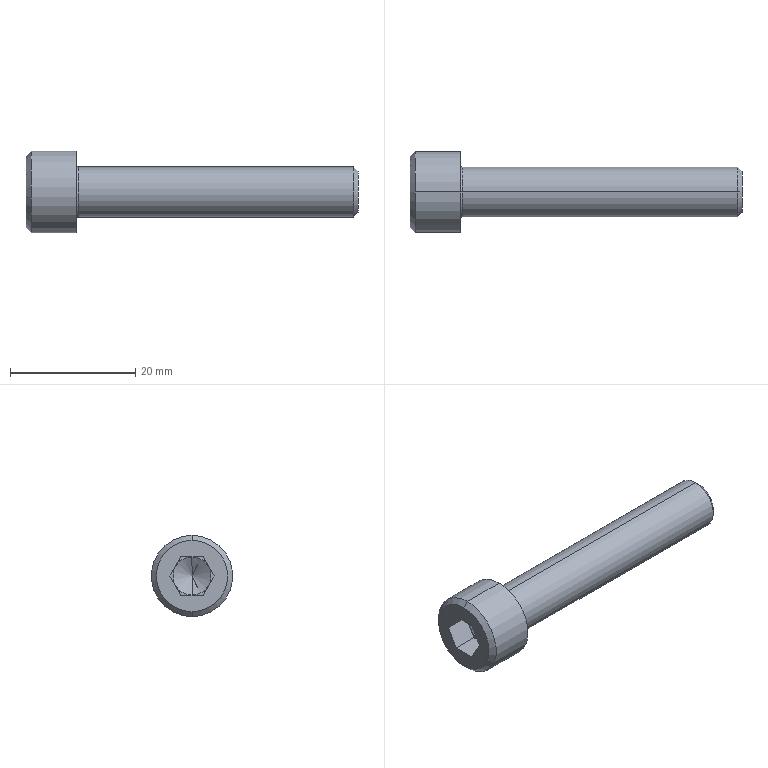Part | SolidWorks | features CirPattern 3, Cut 3, RevCut 2, Fillet 1, LPattern 1, Revolution 1 | 1 solid | 27 faces | box 53 x 13 x 13 mm | volume 3161 mm3 | plane 15 | cone 6 | cylinder 4 | torus 2 | commonest cylinder face diameters 8 x2 13 x2
STEP:
#1=CARTESIAN_POINT('',(5.759,0.,0.));
#2=VERTEX_POINT('',#1);
#3=CARTESIAN_POINT('',(4.,0.,3.047));
#4=VERTEX_POINT('',#3);
#5=CARTESIAN_POINT('',(4.,0.,3.048));
#6=DIRECTION('',(-0.5,0.,0.866));
#7=VECTOR('',#6,1000.);
#8=LINE('',#5,#7);
#9=EDGE_CURVE('',#2,#4,#8,.T.);
#10=ORIENTED_EDGE('',*,*,#9,.F.);
#11=CARTESIAN_POINT('',(4.,0.,-3.047));
#12=VERTEX_POINT('',#11);
#13=CARTESIAN_POINT('',(4.,0.,-3.048));
#14=DIRECTION('',(-0.5,0.,-0.866));
#15=VECTOR('',#14,1000.);
#16=LINE('',#13,#15);
#17=EDGE_CURVE('',#2,#12,#16,.T.);
#18=ORIENTED_EDGE('',*,*,#17,.T.);
#19=CARTESIAN_POINT('',(4.,-2.639,-1.524));
#20=VERTEX_POINT('',#19);
#21=CARTESIAN_POINT('',(4.,0.,0.));
#22=DIRECTION('',(-1.,0.,0.));
#23=DIRECTION('',(0.,0.,1.));
#24=AXIS2_PLACEMENT_3D('',#21,#22,#23);
#25=CIRCLE('',#24,3.048);
#26=EDGE_CURVE('',#12,#20,#25,.T.);
#27=ORIENTED_EDGE('',*,*,#26,.T.);
#28=CARTESIAN_POINT('',(4.,-2.639,1.524));
#29=VERTEX_POINT('',#28);
#30=CARTESIAN_POINT('',(4.,0.,0.));
#31=DIRECTION('',(-1.,0.,0.));
#32=DIRECTION('',(0.,0.,1.));
#33=AXIS2_PLACEMENT_3D('',#30,#31,#32);
#34=CIRCLE('',#33,3.048);
#35=EDGE_CURVE('',#20,#29,#34,.T.);
#36=ORIENTED_EDGE('',*,*,#35,.T.);
#37=CARTESIAN_POINT('',(4.,0.,0.));
#38=DIRECTION('',(-1.,0.,0.));
#39=DIRECTION('',(0.,0.,1.));
#40=AXIS2_PLACEMENT_3D('',#37,#38,#39);
#41=CIRCLE('',#40,3.048);
#42=EDGE_CURVE('',#29,#4,#41,.T.);
#43=ORIENTED_EDGE('',*,*,#42,.T.);
#44=EDGE_LOOP('',(#10,#18,#27,#36,#43));
#45=FACE_OUTER_BOUND('',#44,.T.);
#46=CARTESIAN_POINT('',(4.,0.,0.));
#47=DIRECTION('',(-1.,0.,0.));
#48=DIRECTION('',(0.,0.,1.));
#49=AXIS2_PLACEMENT_3D('',#46,#47,#48);
#50=CONICAL_SURFACE('',#49,3.048,1.047);
#51=ADVANCED_FACE('',(#45),#50,.F.);
#52=CARTESIAN_POINT('',(8.4,0.,4.));
#53=VERTEX_POINT('',#52);
#54=CARTESIAN_POINT('',(8.4,0.,-4.));
#55=VERTEX_POINT('',#54);
#56=CARTESIAN_POINT('',(8.4,0.,0.));
#57=DIRECTION('',(1.,0.,0.));
#58=DIRECTION('',(0.,0.,-1.));
#59=AXIS2_PLACEMENT_3D('',#56,#57,#58);
#60=CIRCLE('',#59,4.);
#61=EDGE_CURVE('',#53,#55,#60,.T.);
#62=ORIENTED_EDGE('',*,*,#61,.F.);
#63=CARTESIAN_POINT('',(8.,0.,4.4));
#64=VERTEX_POINT('',#63);
#65=CARTESIAN_POINT('',(8.4,0.,4.4));
#66=DIRECTION('',(0.,1.,0.));
#67=DIRECTION('',(0.,0.,1.));
#68=AXIS2_PLACEMENT_3D('',#65,#66,#67);
#69=CIRCLE('',#68,0.4);
#70=EDGE_CURVE('',#53,#64,#69,.T.);
#71=ORIENTED_EDGE('',*,*,#70,.T.);
#72=CARTESIAN_POINT('',(8.,0.,-4.4));
#73=VERTEX_POINT('',#72);
#74=CARTESIAN_POINT('',(8.,0.,0.));
#75=DIRECTION('',(-1.,0.,0.));
#76=DIRECTION('',(0.,0.,-1.));
#77=AXIS2_PLACEMENT_3D('',#74,#75,#76);
#78=CIRCLE('',#77,4.4);
#79=EDGE_CURVE('',#73,#64,#78,.T.);
#80=ORIENTED_EDGE('',*,*,#79,.F.);
#81=CARTESIAN_POINT('',(8.4,0.,-4.4));
#82=DIRECTION('',(0.,-1.,0.));
#83=DIRECTION('',(0.,0.,-1.));
#84=AXIS2_PLACEMENT_3D('',#81,#82,#83);
#85=CIRCLE('',#84,0.4);
#86=EDGE_CURVE('',#55,#73,#85,.T.);
#87=ORIENTED_EDGE('',*,*,#86,.F.);
#88=EDGE_LOOP('',(#62,#71,#80,#87));
#89=FACE_OUTER_BOUND('',#88,.T.);
#90=CARTESIAN_POINT('',(8.4,0.,0.));
#91=DIRECTION('',(1.,0.,0.));
#92=DIRECTION('',(0.,0.,-1.));
#93=AXIS2_PLACEMENT_3D('',#90,#91,#92);
#94=TOROIDAL_SURFACE('',#93,4.4,0.4);
#95=ADVANCED_FACE('',(#89),#94,.F.);
#96=CARTESIAN_POINT('',(0.,0.,5.7));
#97=VERTEX_POINT('',#96);
#98=CARTESIAN_POINT('',(0.,0.,-5.7));
#99=VERTEX_POINT('',#98);
#100=CARTESIAN_POINT('',(0.,0.,0.));
#101=DIRECTION('',(-1.,0.,0.));
#102=DIRECTION('',(0.,0.,1.));
#103=AXIS2_PLACEMENT_3D('',#100,#101,#102);
#104=CIRCLE('',#103,5.7);
#105=EDGE_CURVE('',#97,#99,#104,.T.);
#106=ORIENTED_EDGE('',*,*,#105,.F.);
#107=CARTESIAN_POINT('',(0.8,0.,6.5));
#108=VERTEX_POINT('',#107);
#109=CARTESIAN_POINT('',(0.,0.,5.7));
#110=DIRECTION('',(0.7071,0.,0.7071));
#111=VECTOR('',#110,1000.);
#112=LINE('',#109,#111);
#113=EDGE_CURVE('',#97,#108,#112,.T.);
#114=ORIENTED_EDGE('',*,*,#113,.T.);
#115=CARTESIAN_POINT('',(0.8,0.,-6.5));
#116=VERTEX_POINT('',#115);
#117=CARTESIAN_POINT('',(0.8,0.,0.));
#118=DIRECTION('',(-1.,0.,0.));
#119=DIRECTION('',(0.,0.,1.));
#120=AXIS2_PLACEMENT_3D('',#117,#118,#119);
#121=CIRCLE('',#120,6.5);
#122=EDGE_CURVE('',#108,#116,#121,.T.);
#123=ORIENTED_EDGE('',*,*,#122,.T.);
#124=CARTESIAN_POINT('',(0.,0.,-5.7));
#125=DIRECTION('',(0.7071,0.,-0.7071));
#126=VECTOR('',#125,1000.);
#127=LINE('',#124,#126);
#128=EDGE_CURVE('',#99,#116,#127,.T.);
#129=ORIENTED_EDGE('',*,*,#128,.F.);
#130=EDGE_LOOP('',(#106,#114,#123,#129));
#131=FACE_OUTER_BOUND('',#130,.T.);
#132=CARTESIAN_POINT('',(0.,0.,0.));
#133=DIRECTION('',(1.,0.,0.));
#134=DIRECTION('',(0.,0.,-1.));
#135=AXIS2_PLACEMENT_3D('',#132,#133,#134);
#136=CONICAL_SURFACE('',#135,5.7,0.7854);
#137=ADVANCED_FACE('',(#131),#136,.T.);
#138=CARTESIAN_POINT('',(8.,0.,6.5));
#139=VERTEX_POINT('',#138);
#140=CARTESIAN_POINT('',(8.,0.,-6.5));
#141=VERTEX_POINT('',#140);
#142=CARTESIAN_POINT('',(8.,0.,0.));
#143=DIRECTION('',(-1.,0.,0.));
#144=DIRECTION('',(0.,0.,1.));
#145=AXIS2_PLACEMENT_3D('',#142,#143,#144);
#146=CIRCLE('',#145,6.5);
#147=EDGE_CURVE('',#139,#141,#146,.T.);
#148=ORIENTED_EDGE('',*,*,#147,.T.);
#149=CARTESIAN_POINT('',(-31.75,0.,-6.5));
#150=DIRECTION('',(-1.,0.,0.));
#151=VECTOR('',#150,1000.);
#152=LINE('',#149,#151);
#153=EDGE_CURVE('',#141,#116,#152,.T.);
#154=ORIENTED_EDGE('',*,*,#153,.T.);
#155=ORIENTED_EDGE('',*,*,#122,.F.);
#156=CARTESIAN_POINT('',(-31.75,0.,6.5));
#157=DIRECTION('',(-1.,0.,0.));
#158=VECTOR('',#157,1000.);
#159=LINE('',#156,#158);
#160=EDGE_CURVE('',#139,#108,#159,.T.);
#161=ORIENTED_EDGE('',*,*,#160,.F.);
#162=EDGE_LOOP('',(#148,#154,#155,#161));
#163=FACE_OUTER_BOUND('',#162,.T.);
#164=CARTESIAN_POINT('',(-31.75,0.,0.));
#165=DIRECTION('',(-1.,0.,0.));
#166=DIRECTION('',(0.,0.,1.));
#167=AXIS2_PLACEMENT_3D('',#164,#165,#166);
#168=CYLINDRICAL_SURFACE('',#167,6.5);
#169=ADVANCED_FACE('',(#163),#168,.T.);
#170=CARTESIAN_POINT('',(52.31,0.,4.));
#171=VERTEX_POINT('',#170);
#172=CARTESIAN_POINT('',(52.31,0.,-4.));
#173=VERTEX_POINT('',#172);
#174=CARTESIAN_POINT('',(52.31,0.,0.));
#175=DIRECTION('',(-1.,0.,0.));
#176=DIRECTION('',(0.,0.,1.));
#177=AXIS2_PLACEMENT_3D('',#174,#175,#176);
#178=CIRCLE('',#177,4.);
#179=EDGE_CURVE('',#171,#173,#178,.T.);
#180=ORIENTED_EDGE('',*,*,#179,.T.);
#181=CARTESIAN_POINT('',(-31.75,0.,-4.));
#182=DIRECTION('',(-1.,0.,0.));
#183=VECTOR('',#182,1000.);
#184=LINE('',#181,#183);
#185=EDGE_CURVE('',#173,#55,#184,.T.);
#186=ORIENTED_EDGE('',*,*,#185,.T.);
#187=CARTESIAN_POINT('',(8.4,0.,0.));
#188=DIRECTION('',(1.,0.,0.));
#189=DIRECTION('',(0.,0.,-1.));
#190=AXIS2_PLACEMENT_3D('',#187,#188,#189);
#191=CIRCLE('',#190,4.);
#192=EDGE_CURVE('',#55,#53,#191,.T.);
#193=ORIENTED_EDGE('',*,*,#192,.T.);
#194=CARTESIAN_POINT('',(-31.75,0.,4.));
#195=DIRECTION('',(-1.,0.,0.));
#196=VECTOR('',#195,1000.);
#197=LINE('',#194,#196);
#198=EDGE_CURVE('',#171,#53,#197,.T.);
#199=ORIENTED_EDGE('',*,*,#198,.F.);
#200=EDGE_LOOP('',(#180,#186,#193,#199));
#201=FACE_OUTER_BOUND('',#200,.T.);
#202=CARTESIAN_POINT('',(-31.75,0.,0.));
#203=DIRECTION('',(-1.,0.,0.));
#204=DIRECTION('',(0.,0.,1.));
#205=AXIS2_PLACEMENT_3D('',#202,#203,#204);
#206=CYLINDRICAL_SURFACE('',#205,4.);
#207=ADVANCED_FACE('',(#201),#206,.T.);
#208=CARTESIAN_POINT('',(53.,0.,3.309));
#209=VERTEX_POINT('',#208);
#210=CARTESIAN_POINT('',(53.,0.,-3.309));
#211=VERTEX_POINT('',#210);
#212=CARTESIAN_POINT('',(53.,0.,0.));
#213=DIRECTION('',(-1.,0.,0.));
#214=DIRECTION('',(0.,0.,1.));
#215=AXIS2_PLACEMENT_3D('',#212,#213,#214);
#216=CIRCLE('',#215,3.309);
#217=EDGE_CURVE('',#209,#211,#216,.T.);
#218=ORIENTED_EDGE('',*,*,#217,.T.);
#219=CARTESIAN_POINT('',(53.,0.,-3.309));
#220=DIRECTION('',(-0.7071,0.,-0.7071));
#221=VECTOR('',#220,1000.);
#222=LINE('',#219,#221);
#223=EDGE_CURVE('',#211,#173,#222,.T.);
#224=ORIENTED_EDGE('',*,*,#223,.T.);
#225=ORIENTED_EDGE('',*,*,#179,.F.);
#226=CARTESIAN_POINT('',(53.,0.,3.309));
#227=DIRECTION('',(-0.7071,0.,0.7071));
#228=VECTOR('',#227,1000.);
#229=LINE('',#226,#228);
#230=EDGE_CURVE('',#209,#171,#229,.T.);
#231=ORIENTED_EDGE('',*,*,#230,.F.);
#232=EDGE_LOOP('',(#218,#224,#225,#231));
#233=FACE_OUTER_BOUND('',#232,.T.);
#234=CARTESIAN_POINT('',(53.,0.,0.));
#235=DIRECTION('',(-1.,0.,0.));
#236=DIRECTION('',(0.,0.,1.));
#237=AXIS2_PLACEMENT_3D('',#234,#235,#236);
#238=CONICAL_SURFACE('',#237,3.309,0.7854);
#239=ADVANCED_FACE('',(#233),#238,.T.);
#240=CARTESIAN_POINT('',(0.,3.519,0.));
#241=VERTEX_POINT('',#240);
#242=CARTESIAN_POINT('',(0.,1.759,3.047));
#243=VERTEX_POINT('',#242);
#244=CARTESIAN_POINT('',(0.,3.519,0.));
#245=DIRECTION('',(0.,-0.5,0.866));
#246=VECTOR('',#245,1000.);
#247=LINE('',#244,#246);
#248=EDGE_CURVE('',#241,#243,#247,.T.);
#249=ORIENTED_EDGE('',*,*,#248,.T.);
#250=CARTESIAN_POINT('',(0.,-1.759,3.048));
#251=VERTEX_POINT('',#250);
#252=CARTESIAN_POINT('',(0.,-1.759,3.048));
#253=DIRECTION('',(0.,1.,0.));
#254=VECTOR('',#253,1000.);
#255=LINE('',#252,#254);
#256=EDGE_CURVE('',#251,#243,#255,.T.);
#257=ORIENTED_EDGE('',*,*,#256,.F.);
#258=CARTESIAN_POINT('',(0.,-3.519,0.));
#259=VERTEX_POINT('',#258);
#260=CARTESIAN_POINT('',(0.,-1.759,3.048));
#261=DIRECTION('',(0.,-0.5,-0.866));
#262=VECTOR('',#261,1000.);
#263=LINE('',#260,#262);
#264=EDGE_CURVE('',#251,#259,#263,.T.);
#265=ORIENTED_EDGE('',*,*,#264,.T.);
#266=CARTESIAN_POINT('',(0.,-1.759,-3.047));
#267=VERTEX_POINT('',#266);
#268=CARTESIAN_POINT('',(0.,-3.519,0.));
#269=DIRECTION('',(0.,0.5,-0.866));
#270=VECTOR('',#269,1000.);
#271=LINE('',#268,#270);
#272=EDGE_CURVE('',#259,#267,#271,.T.);
#273=ORIENTED_EDGE('',*,*,#272,.T.);
#274=CARTESIAN_POINT('',(0.,1.759,-3.048));
#275=VERTEX_POINT('',#274);
#276=CARTESIAN_POINT('',(0.,1.759,-3.048));
#277=DIRECTION('',(0.,-1.,0.));
#278=VECTOR('',#277,1000.);
#279=LINE('',#276,#278);
#280=EDGE_CURVE('',#275,#267,#279,.T.);
#281=ORIENTED_EDGE('',*,*,#280,.F.);
#282=CARTESIAN_POINT('',(0.,3.519,0.));
#283=DIRECTION('',(0.,-0.5,-0.866));
#284=VECTOR('',#283,1000.);
#285=LINE('',#282,#284);
#286=EDGE_CURVE('',#241,#275,#285,.T.);
#287=ORIENTED_EDGE('',*,*,#286,.F.);
#288=EDGE_LOOP('',(#249,#257,#265,#273,#281,#287));
#289=FACE_BOUND('',#288,.T.);
#290=CARTESIAN_POINT('',(0.,0.,0.));
#291=DIRECTION('',(-1.,0.,0.));
#292=DIRECTION('',(0.,0.,1.));
#293=AXIS2_PLACEMENT_3D('',#290,#291,#292);
#294=CIRCLE('',#293,5.7);
#295=EDGE_CURVE('',#99,#97,#294,.T.);
#296=ORIENTED_EDGE('',*,*,#295,.T.);
#297=ORIENTED_EDGE('',*,*,#105,.T.);
#298=EDGE_LOOP('',(#296,#297));
#299=FACE_OUTER_BOUND('',#298,.T.);
#300=CARTESIAN_POINT('',(0.,0.,0.));
#301=DIRECTION('',(-1.,0.,0.));
#302=DIRECTION('',(0.,0.,1.));
#303=AXIS2_PLACEMENT_3D('',#300,#301,#302);
#304=PLANE('',#303);
#305=ADVANCED_FACE('',(#289,#299),#304,.T.);
#306=ORIENTED_EDGE('',*,*,#217,.F.);
#307=CARTESIAN_POINT('',(53.,0.,0.));
#308=DIRECTION('',(-1.,0.,0.));
#309=DIRECTION('',(0.,0.,1.));
#310=AXIS2_PLACEMENT_3D('',#307,#308,#309);
#311=CIRCLE('',#310,3.309);
#312=EDGE_CURVE('',#211,#209,#311,.T.);
#313=ORIENTED_EDGE('',*,*,#312,.F.);
#314=EDGE_LOOP('',(#306,#313));
#315=FACE_OUTER_BOUND('',#314,.T.);
#316=CARTESIAN_POINT('',(53.,3.309,0.));
#317=DIRECTION('',(1.,0.,0.));
#318=DIRECTION('',(0.,0.,-1.));
#319=AXIS2_PLACEMENT_3D('',#316,#317,#318);
#320=PLANE('',#319);
#321=ADVANCED_FACE('',(#315),#320,.T.);
#322=ORIENTED_EDGE('',*,*,#223,.F.);
#323=ORIENTED_EDGE('',*,*,#312,.T.);
#324=ORIENTED_EDGE('',*,*,#230,.T.);
#325=CARTESIAN_POINT('',(52.31,0.,0.));
#326=DIRECTION('',(-1.,0.,0.));
#327=DIRECTION('',(0.,0.,1.));
#328=AXIS2_PLACEMENT_3D('',#325,#326,#327);
#329=CIRCLE('',#328,4.);
#330=EDGE_CURVE('',#173,#171,#329,.T.);
#331=ORIENTED_EDGE('',*,*,#330,.F.);
#332=EDGE_LOOP('',(#322,#323,#324,#331));
#333=FACE_OUTER_BOUND('',#332,.T.);
#334=CARTESIAN_POINT('',(53.,0.,0.));
#335=DIRECTION('',(-1.,0.,0.));
#336=DIRECTION('',(0.,0.,1.));
#337=AXIS2_PLACEMENT_3D('',#334,#335,#336);
#338=CONICAL_SURFACE('',#337,3.309,0.7854);
#339=ADVANCED_FACE('',(#333),#338,.T.);
#340=ORIENTED_EDGE('',*,*,#185,.F.);
#341=ORIENTED_EDGE('',*,*,#330,.T.);
#342=ORIENTED_EDGE('',*,*,#198,.T.);
#343=ORIENTED_EDGE('',*,*,#61,.T.);
#344=EDGE_LOOP('',(#340,#341,#342,#343));
#345=FACE_OUTER_BOUND('',#344,.T.);
#346=CARTESIAN_POINT('',(-31.75,0.,0.));
#347=DIRECTION('',(-1.,0.,0.));
#348=DIRECTION('',(0.,0.,1.));
#349=AXIS2_PLACEMENT_3D('',#346,#347,#348);
#350=CYLINDRICAL_SURFACE('',#349,4.);
#351=ADVANCED_FACE('',(#345),#350,.T.);
#352=ORIENTED_EDGE('',*,*,#79,.T.);
#353=CARTESIAN_POINT('',(8.,0.,0.));
#354=DIRECTION('',(-1.,0.,0.));
#355=DIRECTION('',(0.,0.,-1.));
#356=AXIS2_PLACEMENT_3D('',#353,#354,#355);
#357=CIRCLE('',#356,4.4);
#358=EDGE_CURVE('',#64,#73,#357,.T.);
#359=ORIENTED_EDGE('',*,*,#358,.T.);
#360=EDGE_LOOP('',(#352,#359));
#361=FACE_BOUND('',#360,.T.);
#362=ORIENTED_EDGE('',*,*,#147,.F.);
#363=CARTESIAN_POINT('',(8.,0.,0.));
#364=DIRECTION('',(-1.,0.,0.));
#365=DIRECTION('',(0.,0.,1.));
#366=AXIS2_PLACEMENT_3D('',#363,#364,#365);
#367=CIRCLE('',#366,6.5);
#368=EDGE_CURVE('',#141,#139,#367,.T.);
#369=ORIENTED_EDGE('',*,*,#368,.F.);
#370=EDGE_LOOP('',(#362,#369));
#371=FACE_OUTER_BOUND('',#370,.T.);
#372=CARTESIAN_POINT('',(8.,6.5,0.));
#373=DIRECTION('',(1.,0.,0.));
#374=DIRECTION('',(0.,0.,-1.));
#375=AXIS2_PLACEMENT_3D('',#372,#373,#374);
#376=PLANE('',#375);
#377=ADVANCED_FACE('',(#361,#371),#376,.T.);
#378=ORIENTED_EDGE('',*,*,#153,.F.);
#379=ORIENTED_EDGE('',*,*,#368,.T.);
#380=ORIENTED_EDGE('',*,*,#160,.T.);
#381=CARTESIAN_POINT('',(0.8,0.,0.));
#382=DIRECTION('',(-1.,0.,0.));
#383=DIRECTION('',(0.,0.,1.));
#384=AXIS2_PLACEMENT_3D('',#381,#382,#383);
#385=CIRCLE('',#384,6.5);
#386=EDGE_CURVE('',#116,#108,#385,.T.);
#387=ORIENTED_EDGE('',*,*,#386,.F.);
#388=EDGE_LOOP('',(#378,#379,#380,#387));
#389=FACE_OUTER_BOUND('',#388,.T.);
#390=CARTESIAN_POINT('',(-31.75,0.,0.));
#391=DIRECTION('',(-1.,0.,0.));
#392=DIRECTION('',(0.,0.,1.));
#393=AXIS2_PLACEMENT_3D('',#390,#391,#392);
#394=CYLINDRICAL_SURFACE('',#393,6.5);
#395=ADVANCED_FACE('',(#389),#394,.T.);
#396=ORIENTED_EDGE('',*,*,#113,.F.);
#397=ORIENTED_EDGE('',*,*,#295,.F.);
#398=ORIENTED_EDGE('',*,*,#128,.T.);
#399=ORIENTED_EDGE('',*,*,#386,.T.);
#400=EDGE_LOOP('',(#396,#397,#398,#399));
#401=FACE_OUTER_BOUND('',#400,.T.);
#402=CARTESIAN_POINT('',(0.,0.,0.));
#403=DIRECTION('',(1.,0.,0.));
#404=DIRECTION('',(0.,0.,-1.));
#405=AXIS2_PLACEMENT_3D('',#402,#403,#404);
#406=CONICAL_SURFACE('',#405,5.7,0.7854);
#407=ADVANCED_FACE('',(#401),#406,.T.);
#408=ORIENTED_EDGE('',*,*,#70,.F.);
#409=ORIENTED_EDGE('',*,*,#192,.F.);
#410=ORIENTED_EDGE('',*,*,#86,.T.);
#411=ORIENTED_EDGE('',*,*,#358,.F.);
#412=EDGE_LOOP('',(#408,#409,#410,#411));
#413=FACE_OUTER_BOUND('',#412,.T.);
#414=CARTESIAN_POINT('',(8.4,0.,0.));
#415=DIRECTION('',(1.,0.,0.));
#416=DIRECTION('',(0.,0.,-1.));
#417=AXIS2_PLACEMENT_3D('',#414,#415,#416);
#418=TOROIDAL_SURFACE('',#417,4.4,0.4);
#419=ADVANCED_FACE('',(#413),#418,.F.);
#420=ORIENTED_EDGE('',*,*,#248,.F.);
#421=CARTESIAN_POINT('',(4.,3.519,0.));
#422=VERTEX_POINT('',#421);
#423=CARTESIAN_POINT('',(4.,3.519,0.));
#424=DIRECTION('',(-1.,0.,0.));
#425=VECTOR('',#424,1000.);
#426=LINE('',#423,#425);
#427=EDGE_CURVE('',#422,#241,#426,.T.);
#428=ORIENTED_EDGE('',*,*,#427,.F.);
#429=CARTESIAN_POINT('',(4.,2.639,1.524));
#430=VERTEX_POINT('',#429);
#431=CARTESIAN_POINT('',(4.,3.519,0.));
#432=DIRECTION('',(0.,-0.5,0.866));
#433=VECTOR('',#432,1000.);
#434=LINE('',#431,#433);
#435=EDGE_CURVE('',#422,#430,#434,.T.);
#436=ORIENTED_EDGE('',*,*,#435,.T.);
#437=CARTESIAN_POINT('',(4.,1.759,3.047));
#438=VERTEX_POINT('',#437);
#439=CARTESIAN_POINT('',(4.,3.519,0.));
#440=DIRECTION('',(0.,-0.5,0.866));
#441=VECTOR('',#440,1000.);
#442=LINE('',#439,#441);
#443=EDGE_CURVE('',#430,#438,#442,.T.);
#444=ORIENTED_EDGE('',*,*,#443,.T.);
#445=CARTESIAN_POINT('',(4.,1.759,3.047));
#446=DIRECTION('',(-1.,0.,0.));
#447=VECTOR('',#446,1000.);
#448=LINE('',#445,#447);
#449=EDGE_CURVE('',#438,#243,#448,.T.);
#450=ORIENTED_EDGE('',*,*,#449,.T.);
#451=EDGE_LOOP('',(#420,#428,#436,#444,#450));
#452=FACE_OUTER_BOUND('',#451,.T.);
#453=CARTESIAN_POINT('',(4.,3.519,0.));
#454=DIRECTION('',(0.,-0.866,-0.5));
#455=DIRECTION('',(0.,0.5,-0.866));
#456=AXIS2_PLACEMENT_3D('',#453,#454,#455);
#457=PLANE('',#456);
#458=ADVANCED_FACE('',(#452),#457,.T.);
#459=ORIENTED_EDGE('',*,*,#256,.T.);
#460=ORIENTED_EDGE('',*,*,#449,.F.);
#461=CARTESIAN_POINT('',(4.,-1.759,3.048));
#462=DIRECTION('',(0.,1.,0.));
#463=VECTOR('',#462,1000.);
#464=LINE('',#461,#463);
#465=EDGE_CURVE('',#4,#438,#464,.T.);
#466=ORIENTED_EDGE('',*,*,#465,.F.);
#467=CARTESIAN_POINT('',(4.,-1.759,3.048));
#468=VERTEX_POINT('',#467);
#469=CARTESIAN_POINT('',(4.,-1.759,3.048));
#470=DIRECTION('',(0.,1.,0.));
#471=VECTOR('',#470,1000.);
#472=LINE('',#469,#471);
#473=EDGE_CURVE('',#468,#4,#472,.T.);
#474=ORIENTED_EDGE('',*,*,#473,.F.);
#475=CARTESIAN_POINT('',(4.,-1.759,3.048));
#476=DIRECTION('',(-1.,0.,0.));
#477=VECTOR('',#476,1000.);
#478=LINE('',#475,#477);
#479=EDGE_CURVE('',#468,#251,#478,.T.);
#480=ORIENTED_EDGE('',*,*,#479,.T.);
#481=EDGE_LOOP('',(#459,#460,#466,#474,#480));
#482=FACE_OUTER_BOUND('',#481,.T.);
#483=CARTESIAN_POINT('',(4.,-1.759,3.048));
#484=DIRECTION('',(0.,0.,1.));
#485=DIRECTION('',(0.,-1.,0.));
#486=AXIS2_PLACEMENT_3D('',#483,#484,#485);
#487=PLANE('',#486);
#488=ADVANCED_FACE('',(#482),#487,.F.);
#489=ORIENTED_EDGE('',*,*,#264,.F.);
#490=ORIENTED_EDGE('',*,*,#479,.F.);
#491=CARTESIAN_POINT('',(4.,-1.759,3.048));
#492=DIRECTION('',(0.,-0.5,-0.866));
#493=VECTOR('',#492,1000.);
#494=LINE('',#491,#493);
#495=EDGE_CURVE('',#468,#29,#494,.T.);
#496=ORIENTED_EDGE('',*,*,#495,.T.);
#497=CARTESIAN_POINT('',(4.,-3.519,0.));
#498=VERTEX_POINT('',#497);
#499=CARTESIAN_POINT('',(4.,-1.759,3.048));
#500=DIRECTION('',(0.,-0.5,-0.866));
#501=VECTOR('',#500,1000.);
#502=LINE('',#499,#501);
#503=EDGE_CURVE('',#29,#498,#502,.T.);
#504=ORIENTED_EDGE('',*,*,#503,.T.);
#505=CARTESIAN_POINT('',(4.,-3.519,0.));
#506=DIRECTION('',(-1.,0.,0.));
#507=VECTOR('',#506,1000.);
#508=LINE('',#505,#507);
#509=EDGE_CURVE('',#498,#259,#508,.T.);
#510=ORIENTED_EDGE('',*,*,#509,.T.);
#511=EDGE_LOOP('',(#489,#490,#496,#504,#510));
#512=FACE_OUTER_BOUND('',#511,.T.);
#513=CARTESIAN_POINT('',(4.,-1.759,3.048));
#514=DIRECTION('',(0.,0.866,-0.5));
#515=DIRECTION('',(0.,0.5,0.866));
#516=AXIS2_PLACEMENT_3D('',#513,#514,#515);
#517=PLANE('',#516);
#518=ADVANCED_FACE('',(#512),#517,.T.);
#519=ORIENTED_EDGE('',*,*,#272,.F.);
#520=ORIENTED_EDGE('',*,*,#509,.F.);
#521=CARTESIAN_POINT('',(4.,-3.519,0.));
#522=DIRECTION('',(0.,0.5,-0.866));
#523=VECTOR('',#522,1000.);
#524=LINE('',#521,#523);
#525=EDGE_CURVE('',#498,#20,#524,.T.);
#526=ORIENTED_EDGE('',*,*,#525,.T.);
#527=CARTESIAN_POINT('',(4.,-1.759,-3.047));
#528=VERTEX_POINT('',#527);
#529=CARTESIAN_POINT('',(4.,-3.519,0.));
#530=DIRECTION('',(0.,0.5,-0.866));
#531=VECTOR('',#530,1000.);
#532=LINE('',#529,#531);
#533=EDGE_CURVE('',#20,#528,#532,.T.);
#534=ORIENTED_EDGE('',*,*,#533,.T.);
#535=CARTESIAN_POINT('',(4.,-1.759,-3.047));
#536=DIRECTION('',(-1.,0.,0.));
#537=VECTOR('',#536,1000.);
#538=LINE('',#535,#537);
#539=EDGE_CURVE('',#528,#267,#538,.T.);
#540=ORIENTED_EDGE('',*,*,#539,.T.);
#541=EDGE_LOOP('',(#519,#520,#526,#534,#540));
#542=FACE_OUTER_BOUND('',#541,.T.);
#543=CARTESIAN_POINT('',(4.,-3.519,0.));
#544=DIRECTION('',(0.,0.866,0.5));
#545=DIRECTION('',(0.,-0.5,0.866));
#546=AXIS2_PLACEMENT_3D('',#543,#544,#545);
#547=PLANE('',#546);
#548=ADVANCED_FACE('',(#542),#547,.T.);
#549=ORIENTED_EDGE('',*,*,#280,.T.);
#550=ORIENTED_EDGE('',*,*,#539,.F.);
#551=CARTESIAN_POINT('',(4.,1.759,-3.048));
#552=DIRECTION('',(0.,-1.,0.));
#553=VECTOR('',#552,1000.);
#554=LINE('',#551,#553);
#555=EDGE_CURVE('',#12,#528,#554,.T.);
#556=ORIENTED_EDGE('',*,*,#555,.F.);
#557=CARTESIAN_POINT('',(4.,1.759,-3.048));
#558=VERTEX_POINT('',#557);
#559=CARTESIAN_POINT('',(4.,1.759,-3.048));
#560=DIRECTION('',(0.,-1.,0.));
#561=VECTOR('',#560,1000.);
#562=LINE('',#559,#561);
#563=EDGE_CURVE('',#558,#12,#562,.T.);
#564=ORIENTED_EDGE('',*,*,#563,.F.);
#565=CARTESIAN_POINT('',(4.,1.759,-3.048));
#566=DIRECTION('',(-1.,0.,0.));
#567=VECTOR('',#566,1000.);
#568=LINE('',#565,#567);
#569=EDGE_CURVE('',#558,#275,#568,.T.);
#570=ORIENTED_EDGE('',*,*,#569,.T.);
#571=EDGE_LOOP('',(#549,#550,#556,#564,#570));
#572=FACE_OUTER_BOUND('',#571,.T.);
#573=CARTESIAN_POINT('',(4.,1.759,-3.048));
#574=DIRECTION('',(0.,0.,-1.));
#575=DIRECTION('',(0.,1.,0.));
#576=AXIS2_PLACEMENT_3D('',#573,#574,#575);
#577=PLANE('',#576);
#578=ADVANCED_FACE('',(#572),#577,.F.);
#579=ORIENTED_EDGE('',*,*,#286,.T.);
#580=ORIENTED_EDGE('',*,*,#569,.F.);
#581=CARTESIAN_POINT('',(4.,2.639,-1.524));
#582=VERTEX_POINT('',#581);
#583=CARTESIAN_POINT('',(4.,3.519,0.));
#584=DIRECTION('',(0.,-0.5,-0.866));
#585=VECTOR('',#584,1000.);
#586=LINE('',#583,#585);
#587=EDGE_CURVE('',#582,#558,#586,.T.);
#588=ORIENTED_EDGE('',*,*,#587,.F.);
#589=CARTESIAN_POINT('',(4.,3.519,0.));
#590=DIRECTION('',(0.,-0.5,-0.866));
#591=VECTOR('',#590,1000.);
#592=LINE('',#589,#591);
#593=EDGE_CURVE('',#422,#582,#592,.T.);
#594=ORIENTED_EDGE('',*,*,#593,.F.);
#595=ORIENTED_EDGE('',*,*,#427,.T.);
#596=EDGE_LOOP('',(#579,#580,#588,#594,#595));
#597=FACE_OUTER_BOUND('',#596,.T.);
#598=CARTESIAN_POINT('',(4.,3.519,0.));
#599=DIRECTION('',(0.,0.866,-0.5));
#600=DIRECTION('',(0.,0.5,0.866));
#601=AXIS2_PLACEMENT_3D('',#598,#599,#600);
#602=PLANE('',#601);
#603=ADVANCED_FACE('',(#597),#602,.F.);
#604=ORIENTED_EDGE('',*,*,#42,.F.);
#605=ORIENTED_EDGE('',*,*,#495,.F.);
#606=ORIENTED_EDGE('',*,*,#473,.T.);
#607=EDGE_LOOP('',(#604,#605,#606));
#608=FACE_OUTER_BOUND('',#607,.T.);
#609=CARTESIAN_POINT('',(4.,1.759,3.047));
#610=DIRECTION('',(-1.,0.,0.));
#611=DIRECTION('',(0.,0.,1.));
#612=AXIS2_PLACEMENT_3D('',#609,#610,#611);
#613=PLANE('',#612);
#614=ADVANCED_FACE('',(#608),#613,.T.);
#615=ORIENTED_EDGE('',*,*,#35,.F.);
#616=ORIENTED_EDGE('',*,*,#525,.F.);
#617=ORIENTED_EDGE('',*,*,#503,.F.);
#618=EDGE_LOOP('',(#615,#616,#617));
#619=FACE_OUTER_BOUND('',#618,.T.);
#620=CARTESIAN_POINT('',(4.,1.759,3.047));
#621=DIRECTION('',(-1.,0.,0.));
#622=DIRECTION('',(0.,0.,1.));
#623=AXIS2_PLACEMENT_3D('',#620,#621,#622);
#624=PLANE('',#623);
#625=ADVANCED_FACE('',(#619),#624,.T.);
#626=ORIENTED_EDGE('',*,*,#26,.F.);
#627=ORIENTED_EDGE('',*,*,#555,.T.);
#628=ORIENTED_EDGE('',*,*,#533,.F.);
#629=EDGE_LOOP('',(#626,#627,#628));
#630=FACE_OUTER_BOUND('',#629,.T.);
#631=CARTESIAN_POINT('',(4.,1.759,3.047));
#632=DIRECTION('',(-1.,0.,0.));
#633=DIRECTION('',(0.,0.,1.));
#634=AXIS2_PLACEMENT_3D('',#631,#632,#633);
#635=PLANE('',#634);
#636=ADVANCED_FACE('',(#630),#635,.T.);
#637=CARTESIAN_POINT('',(4.,0.,0.));
#638=DIRECTION('',(-1.,0.,0.));
#639=DIRECTION('',(0.,0.,1.));
#640=AXIS2_PLACEMENT_3D('',#637,#638,#639);
#641=CIRCLE('',#640,3.048);
#642=EDGE_CURVE('',#582,#12,#641,.T.);
#643=ORIENTED_EDGE('',*,*,#642,.F.);
#644=ORIENTED_EDGE('',*,*,#587,.T.);
#645=ORIENTED_EDGE('',*,*,#563,.T.);
#646=EDGE_LOOP('',(#643,#644,#645));
#647=FACE_OUTER_BOUND('',#646,.T.);
#648=CARTESIAN_POINT('',(4.,1.759,3.047));
#649=DIRECTION('',(-1.,0.,0.));
#650=DIRECTION('',(0.,0.,1.));
#651=AXIS2_PLACEMENT_3D('',#648,#649,#650);
#652=PLANE('',#651);
#653=ADVANCED_FACE('',(#647),#652,.T.);
#654=CARTESIAN_POINT('',(4.,0.,0.));
#655=DIRECTION('',(-1.,0.,0.));
#656=DIRECTION('',(0.,0.,1.));
#657=AXIS2_PLACEMENT_3D('',#654,#655,#656);
#658=CIRCLE('',#657,3.048);
#659=EDGE_CURVE('',#430,#582,#658,.T.);
#660=ORIENTED_EDGE('',*,*,#659,.F.);
#661=ORIENTED_EDGE('',*,*,#435,.F.);
#662=ORIENTED_EDGE('',*,*,#593,.T.);
#663=EDGE_LOOP('',(#660,#661,#662));
#664=FACE_OUTER_BOUND('',#663,.T.);
#665=CARTESIAN_POINT('',(4.,1.759,3.047));
#666=DIRECTION('',(-1.,0.,0.));
#667=DIRECTION('',(0.,0.,1.));
#668=AXIS2_PLACEMENT_3D('',#665,#666,#667);
#669=PLANE('',#668);
#670=ADVANCED_FACE('',(#664),#669,.T.);
#671=CARTESIAN_POINT('',(4.,0.,0.));
#672=DIRECTION('',(-1.,0.,0.));
#673=DIRECTION('',(0.,0.,1.));
#674=AXIS2_PLACEMENT_3D('',#671,#672,#673);
#675=CIRCLE('',#674,3.048);
#676=EDGE_CURVE('',#4,#430,#675,.T.);
#677=ORIENTED_EDGE('',*,*,#676,.F.);
#678=ORIENTED_EDGE('',*,*,#465,.T.);
#679=ORIENTED_EDGE('',*,*,#443,.F.);
#680=EDGE_LOOP('',(#677,#678,#679));
#681=FACE_OUTER_BOUND('',#680,.T.);
#682=CARTESIAN_POINT('',(4.,1.759,3.047));
#683=DIRECTION('',(-1.,0.,0.));
#684=DIRECTION('',(0.,0.,1.));
#685=AXIS2_PLACEMENT_3D('',#682,#683,#684);
#686=PLANE('',#685);
#687=ADVANCED_FACE('',(#681),#686,.T.);
#688=ORIENTED_EDGE('',*,*,#17,.F.);
#689=ORIENTED_EDGE('',*,*,#9,.T.);
#690=ORIENTED_EDGE('',*,*,#676,.T.);
#691=ORIENTED_EDGE('',*,*,#659,.T.);
#692=ORIENTED_EDGE('',*,*,#642,.T.);
#693=EDGE_LOOP('',(#688,#689,#690,#691,#692));
#694=FACE_OUTER_BOUND('',#693,.T.);
#695=CARTESIAN_POINT('',(4.,0.,0.));
#696=DIRECTION('',(-1.,0.,0.));
#697=DIRECTION('',(0.,0.,1.));
#698=AXIS2_PLACEMENT_3D('',#695,#696,#697);
#699=CONICAL_SURFACE('',#698,3.048,1.047);
#700=ADVANCED_FACE('',(#694),#699,.F.);
#701=CLOSED_SHELL('',(#51,#95,#137,#169,#207,#239,#305,#321,#339,#351,#377,#395,#407,#419,#458,#488,#518,#548,#578,#603,#614,#625,#636,#653,#670,#687,#700));
#702=MANIFOLD_SOLID_BREP('',#701);
#703=CARTESIAN_POINT('',(0.,0.,0.));
#704=DIRECTION('',(0.,0.,1.));
#705=DIRECTION('',(1.,0.,0.));
#706=AXIS2_PLACEMENT_3D('',#703,#704,#705);
#707=(LENGTH_UNIT()NAMED_UNIT(*)SI_UNIT(.MILLI.,.METRE.));
#708=UNCERTAINTY_MEASURE_WITH_UNIT(LENGTH_MEASURE(0.00001),#707,'','');
#709=(NAMED_UNIT(*)PLANE_ANGLE_UNIT()SI_UNIT($,.RADIAN.));
#710=(NAMED_UNIT(*)SI_UNIT($,.STERADIAN.)SOLID_ANGLE_UNIT());
#711=(GEOMETRIC_REPRESENTATION_CONTEXT(3)GLOBAL_UNCERTAINTY_ASSIGNED_CONTEXT((#708))GLOBAL_UNIT_ASSIGNED_CONTEXT((#707,#709,#710))REPRESENTATION_CONTEXT('',''));
#712=ADVANCED_BREP_SHAPE_REPRESENTATION('',(#702,#706),#711);